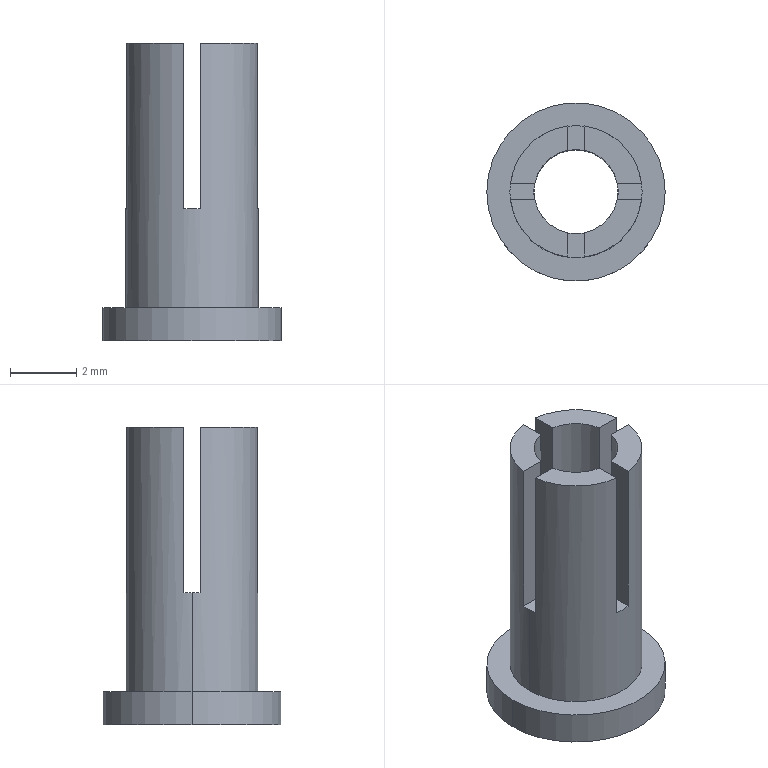Part | STEP file | Glue plug | 1 solid | 24 faces | box 5.4 x 5.4 x 9 mm | volume 70.19 mm3 | plane 18 | cylinder 6 | commonest cylinder face diameters 2.55 x2 4 x2 5.4 x2